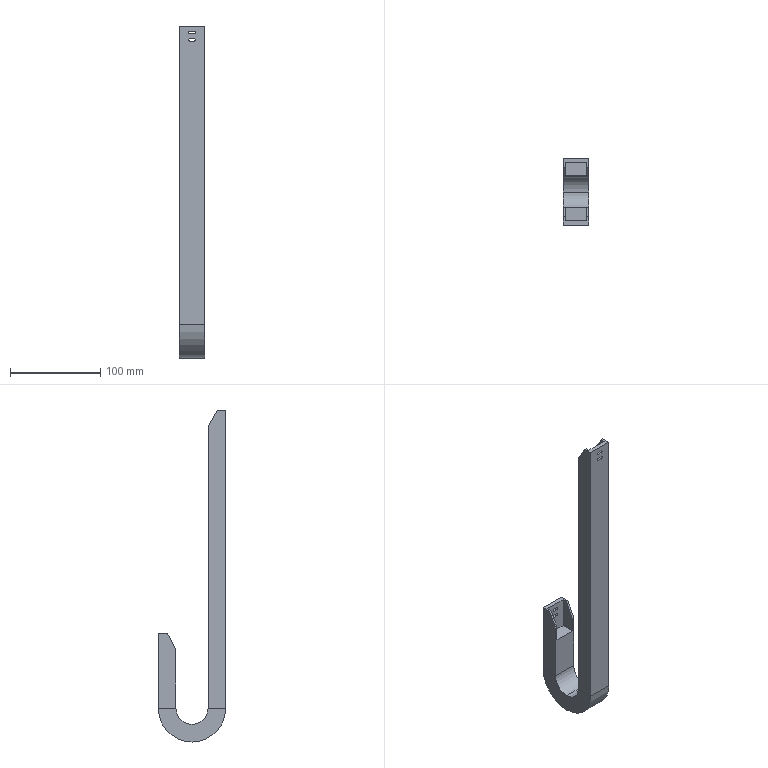Part | STEP file | Cable carrier J15BF.1.20N28 | 1 solid | 44 faces | box 28.5 x 74.5 x 367.25 mm | volume 251972 mm3 | plane 32 | cylinder 12 | commonest cylinder face diameters 3.2 x8 35.5 x2 74.5 x2